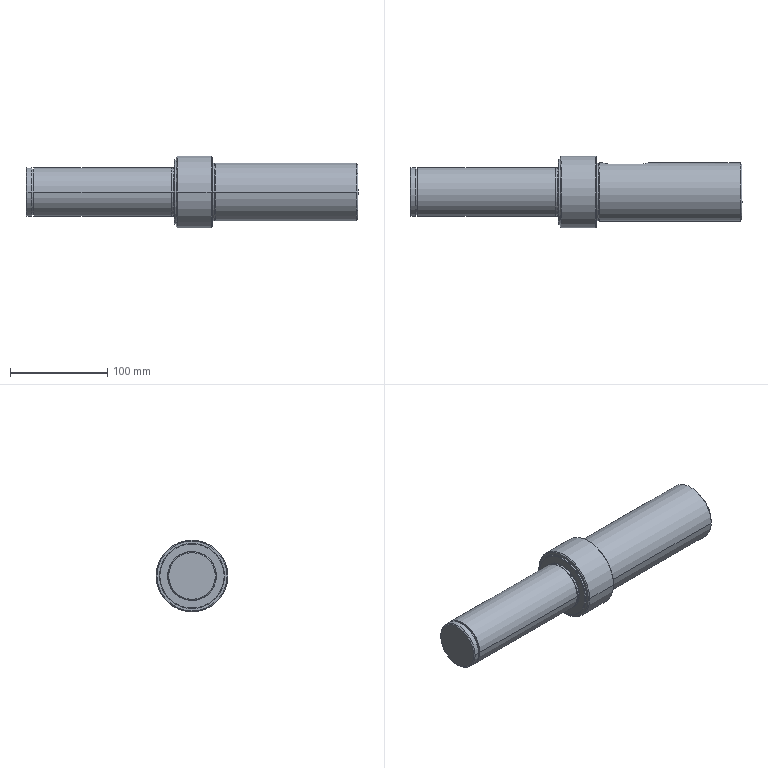Part | SolidWorks | features BaseBody 1 | 1 solid | 56 faces | box 341.34 x 74 x 74 mm | volume 870212 mm3 | cylinder 20 | cone 18 | plane 10 | spline 8 | commonest cylinder face diameters 50 x4 17.294 x2 18 x2 47 x2 49.5 x2 59.5 x2